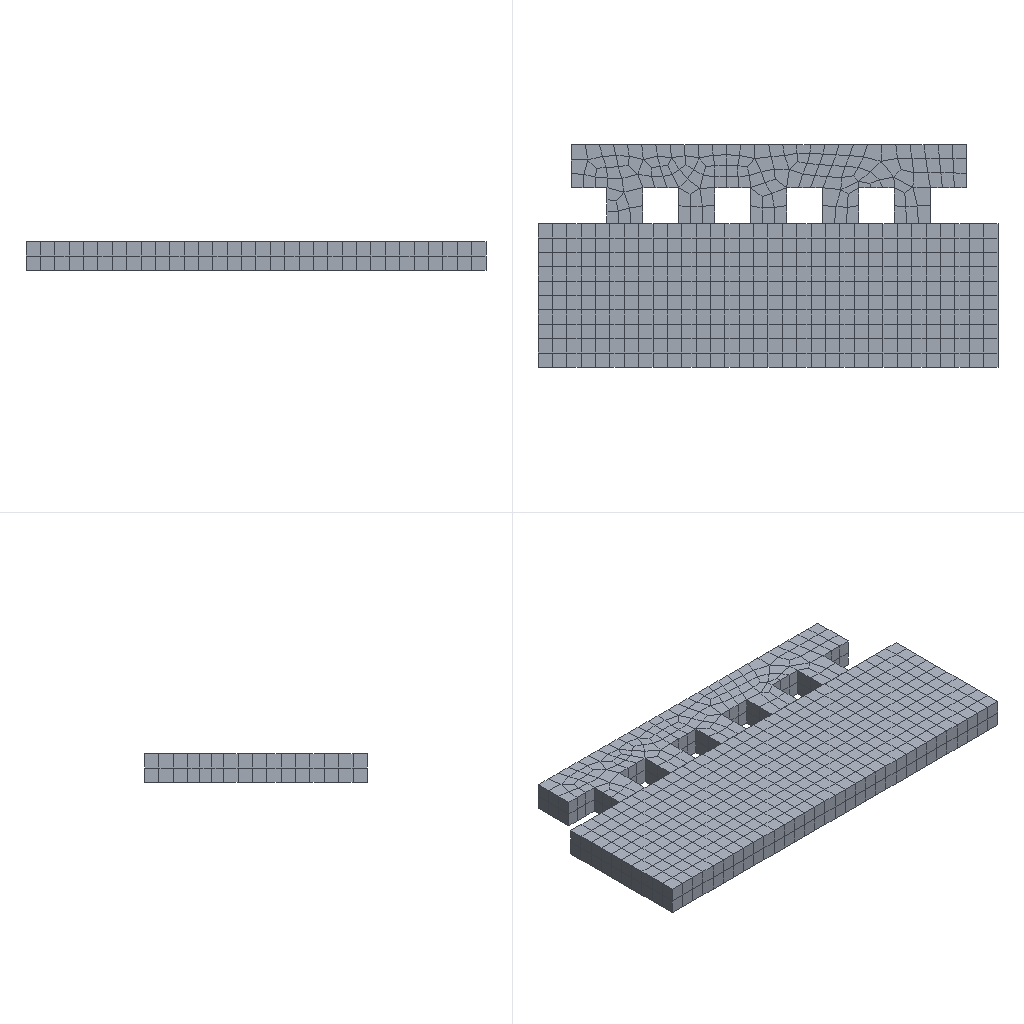Simulation study | abaqus
Set-up summary:
category,name,step,type,value,unit,region
solver,abaqus
solver,version,,,Abaqus/Explicit 2020
units,not stated in the deck,,not stated
analysis,deck,,transient,transient
load_step,Step-1,Step-1,transient
load_step,requested,,,1
mesh,nodes,,,2015
mesh,elements,,,1283
element_type,R3D4,,rigid,353
element_type,C3D8R,,solid,290
element_type,EC3D8R,,solid,640
load,load commands in deck,,count,1
bc,support commands in deck,,count,13
material,MUJU,,in results
material,WATER,,in results
check,setup vs results,,match,"per instance, exact: element labels, types and connectivity; labels of the nodes the elements use; coordinates not compared"
Abaqus input file, long lists of numbers shortened:
*Heading
** Job name: Job-1 Model name: Model-1
** Generated by: Abaqus/CAE 2020
*Preprint, echo=NO, model=NO, history=NO, contact=NO
**
** PARTS
**
*Part, name=muban
*Node
      1, 0.05566, 0.02149,           0.
      2, 0.06941, 0.02149,           0.
** (568 more lines like these left out)
*Element, type=C3D8R
  1, 128, 155, 106, 160, 318, 345, 296, 350
  2,  43,  42, 134, 118, 233, 232, 324, 308
** (288 more lines like these left out)
*Nset, nset=Set-1, generate
   1,  570,    1
*Elset, elset=Set-1, generate
   1,  290,    1
** Section: muban
*Solid Section, elset=Set-1, material=muju
,
*End Part
**
*Part, name=oula
*Node
      1, 0.07521, 0.01511, 0.001
      2, 0.07471, 0.01511, 0.001
** (1087 more lines like these left out)
*Element, type=EC3D8R
  1,  100,  101,  134,  133,    1,    2,   35,   34
  2,  101,  102,  135,  134,    2,    3,   36,   35
** (638 more lines like these left out)
*Nset, nset=Set-1, generate
    1,  1089,     1
*Elset, elset=Set-1, generate
   1,  640,    1
** Section: oula
*Eulerian Section, elset=Set-1
water, water-1
*Surface, type=EULERIAN MATERIAL, name=water-1
water-1
*End Part
**
*Part, name=rig
*Node
      1, 0.01125,           0., 0.001
      2, 0.01125, -0.005, 0.001
** (353 more lines like these left out)
*Element, type=R3D4
 1,   1,  17, 173,  38
 2,  17,  18, 174, 173
** (351 more lines like these left out)
*Node
    356, 0.005625,           0.,           0.
*Nset, nset=rig-RefPt_, internal
356,
*Elset, elset=rig, generate
   1,  353,    1
*End Part
**
**
** ASSEMBLY
**
*Assembly, name=Assembly
**
*Instance, name=muban-1, part=muban
   -0.05527,    -0.02649,           0.
*End Instance
**
*Instance, name=rig-1, part=rig
     0.00125,           0.,           0.
*End Instance
**
*Instance, name=oula-1, part=oula
   -0.05996,    -0.02786,           0.
*End Instance
**
*Nset, nset=Set-1, instance=oula-1
    1,    2,    3,    4,    5,    6,    7,    8,    9,   10,   11,   12,   13,   14,   15,   16
   17,   18,   19,   20,   21,   22,   23,   24,   25,   26,   27,   28,   29,   30,   31,   32
** (44 more lines like these left out)
*Elset, elset=Set-1, instance=oula-1, generate
   1,  640,    1
*Nset, nset=Set-2, instance=oula-1
    1,   33,   34,   66,   67,   99,  100,  132,  133,  165,  166,  198,  199,  231,  232,  264
  265,  297,  298,  330,  331,  363,  364,  396,  397,  429,  430,  462,  463,  495,  496,  528
** (3 more lines like these left out)
*Elset, elset=Set-2, instance=oula-1
   1,  32,  33,  64,  65,  96,  97, 128, 129, 160, 161, 192, 193, 224, 225, 256
 257, 288, 289, 320, 321, 352, 353, 384, 385, 416, 417, 448, 449, 480, 481, 512
** (1 more lines like these left out)
*Nset, nset=Set-3, instance=oula-1, generate
  1,  99,   1
*Elset, elset=Set-3, instance=oula-1, generate
  1,  64,   1
*Nset, nset=Set-4, instance=muban-1
   1,   2,   3,   4,   5,   6,   7,   8,   9,  10,  11,  12,  13,  14,  15,  16
  17,  18,  19,  20,  21,  22,  23,  24,  25,  26,  27,  28,  29,  30,  31,  32
** (22 more lines like these left out)
*Elset, elset=Set-4, instance=muban-1, generate
   1,  290,    1
*Nset, nset=Set-6, instance=rig-1
 356,
*Nset, nset=Set-7, instance=oula-1, generate
    1,  1089,     1
*Elset, elset=Set-7, instance=oula-1, generate
   1,  640,    1
*Nset, nset=_PickedSet14, internal, instance=oula-1, generate
    1,  1089,     1
*Elset, elset=_PickedSet14, internal, instance=oula-1, generate
   1,  640,    1
*Elset, elset=_m_Surf-1_SPOS, internal, instance=rig-1
 23, 24, 25, 26, 93, 94, 95, 96, 97, 98
*Surface, type=ELEMENT, name=m_Surf-1
_m_Surf-1_SPOS, SPOS
*Elset, elset=_s_Surf-1_S3, internal, instance=muban-1
   2,  21,  43,  97, 147, 166, 188, 242
*Elset, elset=_s_Surf-1_S6, internal, instance=muban-1
  13,  20,  22,  28,  40,  83,  87,  89,  91,  92,  94, 158, 165, 167, 173, 185
 228, 232, 234, 236, 237, 239
*Elset, elset=_s_Surf-1_S4, internal, instance=muban-1
  26,  32,  37,  77,  80,  98, 100, 101, 102, 103, 107, 109, 171, 177, 182, 222
 225, 243, 245, 246, 247, 248, 252, 254
*Elset, elset=_s_Surf-1_S5, internal, instance=muban-1
  45, 190
*Surface, type=ELEMENT, name=s_Surf-1
_s_Surf-1_S3, S3
_s_Surf-1_S6, S6
_s_Surf-1_S4, S4
_s_Surf-1_S5, S5
*Rigid Body, ref node=rig-1.rig-RefPt_, elset=rig-1.rig
** Constraint: Constraint-1
*Tie, name=Constraint-1, adjust=yes
s_Surf-1, m_Surf-1
*End Assembly
*Amplitude, name=Amp-1
             0.,              0.,             0.1,              1.
**
** MATERIALS
**
*Material, name=muju
*Density
2000.,
*Elastic
 1e+07, 0.4
*Material, name=water
*Density
1000.,
*Eos, type=USUP
1480.,0.,0.
*Viscosity
 0.001,
**
** INTERACTION PROPERTIES
**
*Surface Interaction, name=IntProp-1
*Friction
 0.2,
*Surface Behavior, pressure-overclosure=HARD
**
** PREDEFINED FIELDS
**
** Name: Predefined Field-1   Type: Material assignment
*Initial Conditions, type=VOLUME FRACTION
Set-7, oula-1.water-1, 1.
** ----------------------------------------------------------------
**
** STEP: Step-1
**
*Step, name=Step-1, nlgeom=YES
*Dynamic, Explicit
, 0.1
*Bulk Viscosity
0.06, 1.2
**
** BOUNDARY CONDITIONS
**
** Name: BC-3 Type: 位移/转角
*Boundary
Set-3, 1, 1
Set-3, 2, 2
Set-3, 3, 3
Set-3, 4, 4
Set-3, 5, 5
Set-3, 6, 6
** Name: BC-4 Type: 位移/转角
*Boundary
Set-4, 3, 3
** Name: BC-5 Type: 位移/转角
*Boundary, amplitude=Amp-1
Set-6, 1, 1
Set-6, 2, 2, -0.0015
Set-6, 3, 3
Set-6, 4, 4
Set-6, 5, 5
Set-6, 6, 6
**
** INTERACTIONS
**
** Interaction: Int-1
*Contact, op=NEW
*Contact Inclusions, ALL EXTERIOR
*Contact Property Assignment
 ,  , IntProp-1
**
** OUTPUT REQUESTS
**
*Restart, write, number interval=1, time marks=NO
**
** FIELD OUTPUT: F-Output-1
**
*Output, field, number interval=50
*Node Output
A, CF, RF, RM, RT, U, V
*Element Output, directions=YES
DENSITY, DENSITYVAVG, E, EACTIVE, EVF, LE, MISES, MISESMAX, MISESONLY, PE, PEEQ, PEEQVAVG, PEVAVG, S, SSAVG, SVAVG
*Contact Output
CDISP, CSTRESS
**
** HISTORY OUTPUT: H-Output-1
**
*Output, history, variable=PRESELECT
*End Step
Results summary:
result,step,Step-1,partial,increments=445772 time=0.078/0.1
result,analysis,,,transient
result,last_loadstep,,,1
result,primary field,,,U
result,reaction total,,FX,-0.001062,model units
result,reaction total,,FY,0.00446,model units
result,reaction total,,FZ,1e-06,model units